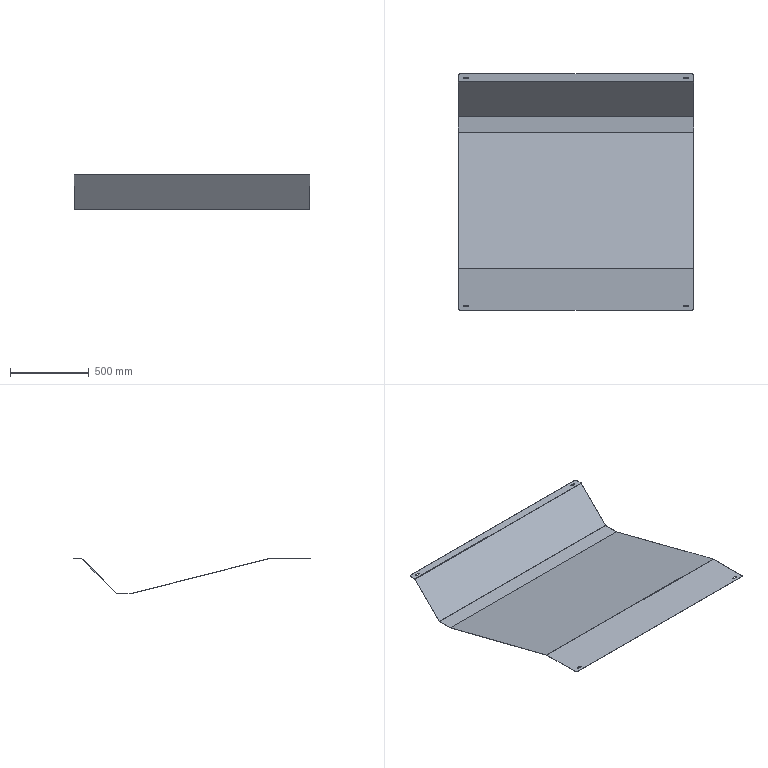Part | SolidWorks | features EdgeFlange 4, Extrusion 1, Fillet 1, FlatPattern 1, ICE 1, SheetMetal 1, SolidToSheetMetal 1 | 1 solid | 62 faces | box 1490 x 1497 x 221.028 mm | volume 3607378 mm3 | plane 38 | cylinder 24 | commonest cylinder face diameters 10 x12 2 x4 5 x4 20 x4